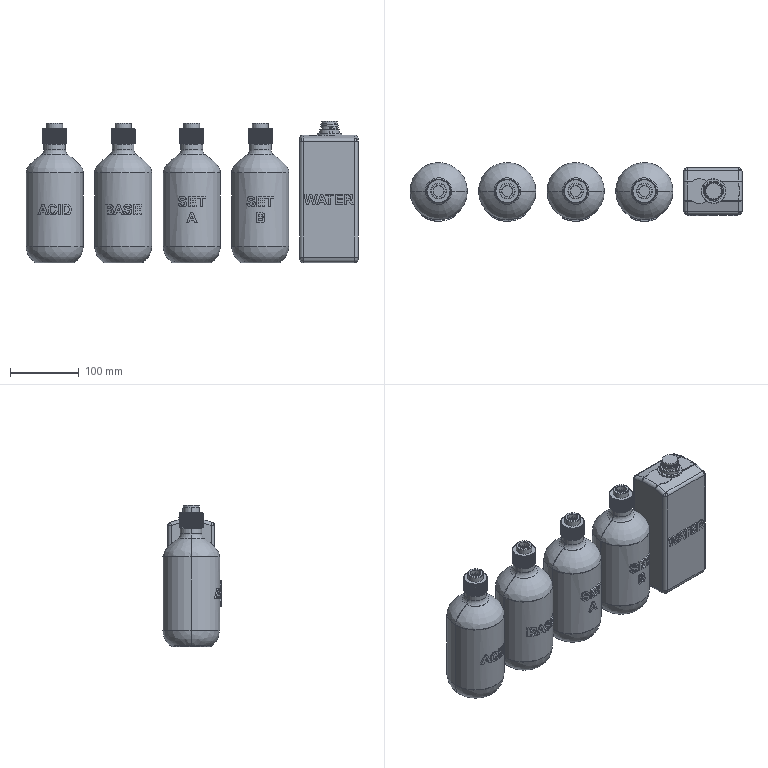Part | SolidWorks | 10 solids | 3842 faces | volume 1269065 mm3 | cylinder 1481 | spline 1100 | sphere 902 | plane 239 | torus 120 | commonest cylinder face diameters 0.3 x880 0.4 x440 83.56 x36 10 x18 15.567 x8 21.567 x8